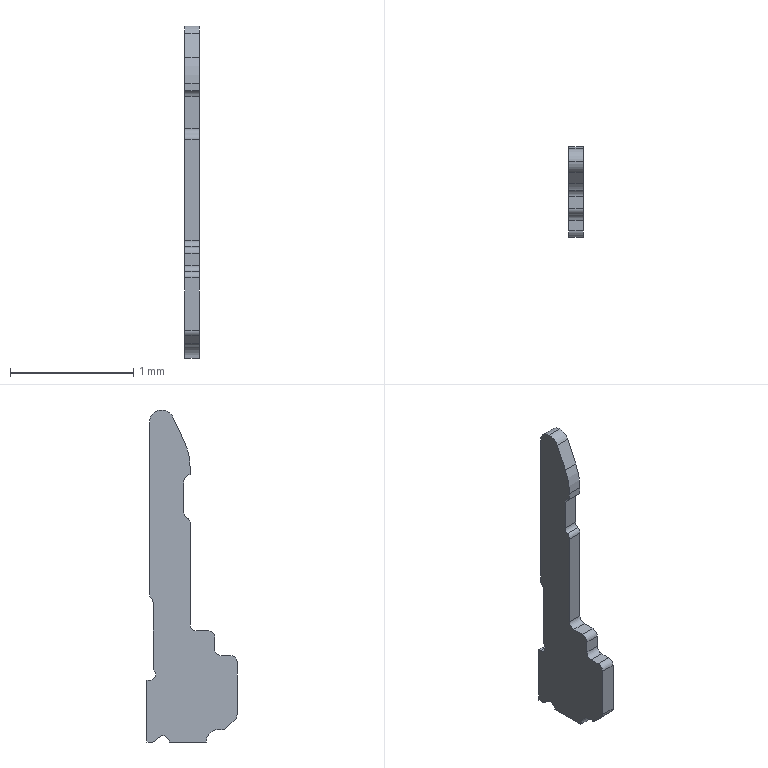Part | Creo | 1 solid | 40 faces | box 0.12 x 0.73 x 2.69 mm | volume 0.132 mm3 | cylinder 20 | plane 20 | commonest cylinder face diameters 0.1 x16 0.2 x3 1 x1
STEP:
#1=CARTESIAN_POINT('',(0.,0.,0.));
#2=DIRECTION('',(0.,0.,1.));
#3=DIRECTION('',(1.,0.,0.));
#4=AXIS2_PLACEMENT_3D('',#1,#2,#3);
#5=CARTESIAN_POINT('',(0.12,978.915,-1855.853));
#6=VERTEX_POINT('',#5);
#7=CARTESIAN_POINT('',(0.12,978.872,-1855.828));
#8=VERTEX_POINT('',#7);
#9=CARTESIAN_POINT('',(0.12,978.872,-1855.878));
#10=DIRECTION('',(1.,0.,0.));
#11=DIRECTION('',(0.,0.866,0.5));
#12=AXIS2_PLACEMENT_3D('',#9,#10,#11);
#13=CIRCLE('',#12,0.05);
#14=EDGE_CURVE('',#6,#8,#13,.T.);
#15=ORIENTED_EDGE('',*,*,#14,.F.);
#16=CARTESIAN_POINT('',(0.,978.915,-1855.853));
#17=VERTEX_POINT('',#16);
#18=CARTESIAN_POINT('',(0.,978.915,-1855.853));
#19=DIRECTION('',(1.,0.,0.));
#20=VECTOR('',#19,0.12);
#21=LINE('',#18,#20);
#22=EDGE_CURVE('',#17,#6,#21,.T.);
#23=ORIENTED_EDGE('',*,*,#22,.F.);
#24=CARTESIAN_POINT('',(0.,978.872,-1855.828));
#25=VERTEX_POINT('',#24);
#26=CARTESIAN_POINT('',(0.,978.872,-1855.878));
#27=DIRECTION('',(-1.,0.,0.));
#28=DIRECTION('',(0.,0.,1.));
#29=AXIS2_PLACEMENT_3D('',#26,#27,#28);
#30=CIRCLE('',#29,0.05);
#31=EDGE_CURVE('',#25,#17,#30,.T.);
#32=ORIENTED_EDGE('',*,*,#31,.F.);
#33=CARTESIAN_POINT('',(0.,978.872,-1855.828));
#34=DIRECTION('',(1.,0.,0.));
#35=VECTOR('',#34,0.12);
#36=LINE('',#33,#35);
#37=EDGE_CURVE('',#25,#8,#36,.T.);
#38=ORIENTED_EDGE('',*,*,#37,.T.);
#39=EDGE_LOOP('',(#15,#23,#32,#38));
#40=FACE_OUTER_BOUND('',#39,.F.);
#41=CARTESIAN_POINT('',(0.12,978.872,-1855.878));
#42=DIRECTION('',(-1.,0.,0.));
#43=DIRECTION('',(0.,0.,1.));
#44=AXIS2_PLACEMENT_3D('',#41,#42,#43);
#45=CYLINDRICAL_SURFACE('',#44,0.05);
#46=ADVANCED_FACE('',(#40),#45,.F.);
#47=CARTESIAN_POINT('',(0.12,978.286,-1855.693));
#48=VERTEX_POINT('',#47);
#49=CARTESIAN_POINT('',(0.12,978.272,-1855.658));
#50=VERTEX_POINT('',#49);
#51=CARTESIAN_POINT('',(0.12,978.322,-1855.658));
#52=DIRECTION('',(-1.,0.,0.));
#53=DIRECTION('',(0.,-0.7071,-0.7071));
#54=AXIS2_PLACEMENT_3D('',#51,#52,#53);
#55=CIRCLE('',#54,0.05);
#56=EDGE_CURVE('',#48,#50,#55,.T.);
#57=ORIENTED_EDGE('',*,*,#56,.T.);
#58=CARTESIAN_POINT('',(0.12,978.272,-1855.228));
#59=VERTEX_POINT('',#58);
#60=CARTESIAN_POINT('',(0.12,978.272,-1855.658));
#61=DIRECTION('',(0.,0.,1.));
#62=VECTOR('',#61,0.4293);
#63=LINE('',#60,#62);
#64=EDGE_CURVE('',#50,#59,#63,.T.);
#65=ORIENTED_EDGE('',*,*,#64,.T.);
#66=CARTESIAN_POINT('',(0.12,978.322,-1855.178));
#67=VERTEX_POINT('',#66);
#68=CARTESIAN_POINT('',(0.12,978.322,-1855.228));
#69=DIRECTION('',(-1.,0.,0.));
#70=DIRECTION('',(0.,-1.,0.));
#71=AXIS2_PLACEMENT_3D('',#68,#69,#70);
#72=CIRCLE('',#71,0.05);
#73=EDGE_CURVE('',#59,#67,#72,.T.);
#74=ORIENTED_EDGE('',*,*,#73,.T.);
#75=CARTESIAN_POINT('',(0.12,978.402,-1855.178));
#76=VERTEX_POINT('',#75);
#77=CARTESIAN_POINT('',(0.12,978.322,-1855.178));
#78=DIRECTION('',(0.,1.,0.));
#79=VECTOR('',#78,0.08);
#80=LINE('',#77,#79);
#81=EDGE_CURVE('',#67,#76,#80,.T.);
#82=ORIENTED_EDGE('',*,*,#81,.T.);
#83=CARTESIAN_POINT('',(0.12,978.452,-1855.128));
#84=VERTEX_POINT('',#83);
#85=CARTESIAN_POINT('',(0.12,978.402,-1855.128));
#86=DIRECTION('',(1.,0.,0.));
#87=DIRECTION('',(0.,0.,-1.));
#88=AXIS2_PLACEMENT_3D('',#85,#86,#87);
#89=CIRCLE('',#88,0.05);
#90=EDGE_CURVE('',#76,#84,#89,.T.);
#91=ORIENTED_EDGE('',*,*,#90,.T.);
#92=CARTESIAN_POINT('',(0.12,978.452,-1855.028));
#93=VERTEX_POINT('',#92);
#94=CARTESIAN_POINT('',(0.12,978.452,-1855.128));
#95=DIRECTION('',(0.,0.,1.));
#96=VECTOR('',#95,0.1);
#97=LINE('',#94,#96);
#98=EDGE_CURVE('',#84,#93,#97,.T.);
#99=ORIENTED_EDGE('',*,*,#98,.T.);
#100=CARTESIAN_POINT('',(0.12,978.502,-1854.978));
#101=VERTEX_POINT('',#100);
#102=CARTESIAN_POINT('',(0.12,978.502,-1855.028));
#103=DIRECTION('',(-1.,0.,0.));
#104=DIRECTION('',(0.,-1.,0.));
#105=AXIS2_PLACEMENT_3D('',#102,#103,#104);
#106=CIRCLE('',#105,0.05);
#107=EDGE_CURVE('',#93,#101,#106,.T.);
#108=ORIENTED_EDGE('',*,*,#107,.T.);
#109=CARTESIAN_POINT('',(0.12,978.602,-1854.978));
#110=VERTEX_POINT('',#109);
#111=CARTESIAN_POINT('',(0.12,978.502,-1854.978));
#112=DIRECTION('',(0.,1.,0.));
#113=VECTOR('',#112,0.1);
#114=LINE('',#111,#113);
#115=EDGE_CURVE('',#101,#110,#114,.T.);
#116=ORIENTED_EDGE('',*,*,#115,.T.);
#117=CARTESIAN_POINT('',(0.12,978.652,-1854.928));
#118=VERTEX_POINT('',#117);
#119=CARTESIAN_POINT('',(0.12,978.602,-1854.928));
#120=DIRECTION('',(1.,0.,0.));
#121=DIRECTION('',(0.,0.,-1.));
#122=AXIS2_PLACEMENT_3D('',#119,#120,#121);
#123=CIRCLE('',#122,0.05);
#124=EDGE_CURVE('',#110,#118,#123,.T.);
#125=ORIENTED_EDGE('',*,*,#124,.T.);
#126=CARTESIAN_POINT('',(0.12,978.652,-1854.108));
#127=VERTEX_POINT('',#126);
#128=CARTESIAN_POINT('',(0.12,978.652,-1854.928));
#129=DIRECTION('',(0.,0.,1.));
#130=VECTOR('',#129,0.82);
#131=LINE('',#128,#130);
#132=EDGE_CURVE('',#118,#127,#131,.T.);
#133=ORIENTED_EDGE('',*,*,#132,.T.);
#134=CARTESIAN_POINT('',(0.12,978.677,-1854.065));
#135=VERTEX_POINT('',#134);
#136=CARTESIAN_POINT('',(0.12,978.702,-1854.108));
#137=DIRECTION('',(-1.,0.,0.));
#138=DIRECTION('',(0.,-1.,0.));
#139=AXIS2_PLACEMENT_3D('',#136,#137,#138);
#140=CIRCLE('',#139,0.05);
#141=EDGE_CURVE('',#127,#135,#140,.T.);
#142=ORIENTED_EDGE('',*,*,#141,.T.);
#143=CARTESIAN_POINT('',(0.12,978.702,-1854.022));
#144=VERTEX_POINT('',#143);
#145=CARTESIAN_POINT('',(0.12,978.652,-1854.022));
#146=DIRECTION('',(1.,0.,0.));
#147=DIRECTION('',(0.,0.5,-0.866));
#148=AXIS2_PLACEMENT_3D('',#145,#146,#147);
#149=CIRCLE('',#148,0.05);
#150=EDGE_CURVE('',#135,#144,#149,.T.);
#151=ORIENTED_EDGE('',*,*,#150,.T.);
#152=CARTESIAN_POINT('',(0.12,978.702,-1853.764));
#153=VERTEX_POINT('',#152);
#154=CARTESIAN_POINT('',(0.12,978.702,-1854.022));
#155=DIRECTION('',(0.,0.,1.));
#156=VECTOR('',#155,0.258);
#157=LINE('',#154,#156);
#158=EDGE_CURVE('',#144,#153,#157,.T.);
#159=ORIENTED_EDGE('',*,*,#158,.T.);
#160=CARTESIAN_POINT('',(0.12,978.652,-1853.714));
#161=VERTEX_POINT('',#160);
#162=CARTESIAN_POINT('',(0.12,978.652,-1853.764));
#163=DIRECTION('',(1.,0.,0.));
#164=DIRECTION('',(0.,1.,0.000000001));
#165=AXIS2_PLACEMENT_3D('',#162,#163,#164);
#166=CIRCLE('',#165,0.05);
#167=EDGE_CURVE('',#153,#161,#166,.T.);
#168=ORIENTED_EDGE('',*,*,#167,.T.);
#169=CARTESIAN_POINT('',(0.12,978.652,-1853.656));
#170=VERTEX_POINT('',#169);
#171=CARTESIAN_POINT('',(0.12,978.652,-1853.714));
#172=DIRECTION('',(0.,0.,1.));
#173=VECTOR('',#172,0.05743);
#174=LINE('',#171,#173);
#175=EDGE_CURVE('',#161,#170,#174,.T.);
#176=ORIENTED_EDGE('',*,*,#175,.T.);
#177=CARTESIAN_POINT('',(0.12,978.698,-1853.445));
#178=VERTEX_POINT('',#177);
#179=CARTESIAN_POINT('',(0.12,979.152,-1853.656));
#180=DIRECTION('',(-1.,0.,0.));
#181=DIRECTION('',(0.,-1.,0.));
#182=AXIS2_PLACEMENT_3D('',#179,#180,#181);
#183=CIRCLE('',#182,0.5);
#184=EDGE_CURVE('',#170,#178,#183,.T.);
#185=ORIENTED_EDGE('',*,*,#184,.T.);
#186=CARTESIAN_POINT('',(0.12,978.791,-1853.247));
#187=VERTEX_POINT('',#186);
#188=CARTESIAN_POINT('',(0.12,978.698,-1853.445));
#189=DIRECTION('',(0.,0.4226,0.9063));
#190=VECTOR('',#189,0.2189);
#191=LINE('',#188,#190);
#192=EDGE_CURVE('',#178,#187,#191,.T.);
#193=ORIENTED_EDGE('',*,*,#192,.T.);
#194=CARTESIAN_POINT('',(0.12,978.882,-1853.189));
#195=VERTEX_POINT('',#194);
#196=CARTESIAN_POINT('',(0.12,978.882,-1853.289));
#197=DIRECTION('',(-1.,0.,0.));
#198=DIRECTION('',(0.,-0.9063,0.4226));
#199=AXIS2_PLACEMENT_3D('',#196,#197,#198);
#200=CIRCLE('',#199,0.1);
#201=EDGE_CURVE('',#187,#195,#200,.T.);
#202=ORIENTED_EDGE('',*,*,#201,.T.);
#203=CARTESIAN_POINT('',(0.12,978.982,-1853.289));
#204=VERTEX_POINT('',#203);
#205=CARTESIAN_POINT('',(0.12,978.882,-1853.289));
#206=DIRECTION('',(-1.,0.,0.));
#207=DIRECTION('',(0.,0.,1.));
#208=AXIS2_PLACEMENT_3D('',#205,#206,#207);
#209=CIRCLE('',#208,0.1);
#210=EDGE_CURVE('',#195,#204,#209,.T.);
#211=ORIENTED_EDGE('',*,*,#210,.T.);
#212=CARTESIAN_POINT('',(0.12,978.982,-1854.678));
#213=VERTEX_POINT('',#212);
#214=CARTESIAN_POINT('',(0.12,978.982,-1853.289));
#215=DIRECTION('',(0.,0.,-1.));
#216=VECTOR('',#215,1.389);
#217=LINE('',#214,#216);
#218=EDGE_CURVE('',#204,#213,#217,.T.);
#219=ORIENTED_EDGE('',*,*,#218,.T.);
#220=CARTESIAN_POINT('',(0.12,978.967,-1854.713));
#221=VERTEX_POINT('',#220);
#222=CARTESIAN_POINT('',(0.12,978.932,-1854.678));
#223=DIRECTION('',(-1.,0.,0.));
#224=DIRECTION('',(0.,1.,0.));
#225=AXIS2_PLACEMENT_3D('',#222,#223,#224);
#226=CIRCLE('',#225,0.05);
#227=EDGE_CURVE('',#213,#221,#226,.T.);
#228=ORIENTED_EDGE('',*,*,#227,.T.);
#229=CARTESIAN_POINT('',(0.12,978.966,-1854.714));
#230=VERTEX_POINT('',#229);
#231=CARTESIAN_POINT('',(0.12,978.967,-1854.713));
#232=DIRECTION('',(0.,-0.7071,-0.7071));
#233=VECTOR('',#232,0.001005);
#234=LINE('',#231,#233);
#235=EDGE_CURVE('',#221,#230,#234,.T.);
#236=ORIENTED_EDGE('',*,*,#235,.T.);
#237=CARTESIAN_POINT('',(0.12,978.952,-1854.749));
#238=VERTEX_POINT('',#237);
#239=CARTESIAN_POINT('',(0.12,979.002,-1854.749));
#240=DIRECTION('',(1.,0.,0.));
#241=DIRECTION('',(0.,-0.7071,0.7071));
#242=AXIS2_PLACEMENT_3D('',#239,#240,#241);
#243=CIRCLE('',#242,0.05);
#244=EDGE_CURVE('',#230,#238,#243,.T.);
#245=ORIENTED_EDGE('',*,*,#244,.T.);
#246=CARTESIAN_POINT('',(0.12,978.952,-1855.267));
#247=VERTEX_POINT('',#246);
#248=CARTESIAN_POINT('',(0.12,978.952,-1854.749));
#249=DIRECTION('',(0.,0.,-1.));
#250=VECTOR('',#249,0.5179);
#251=LINE('',#248,#250);
#252=EDGE_CURVE('',#238,#247,#251,.T.);
#253=ORIENTED_EDGE('',*,*,#252,.T.);
#254=CARTESIAN_POINT('',(0.12,978.945,-1855.292));
#255=VERTEX_POINT('',#254);
#256=CARTESIAN_POINT('',(0.12,978.902,-1855.267));
#257=DIRECTION('',(-1.,0.,0.));
#258=DIRECTION('',(0.,1.,0.));
#259=AXIS2_PLACEMENT_3D('',#256,#257,#258);
#260=CIRCLE('',#259,0.05);
#261=EDGE_CURVE('',#247,#255,#260,.T.);
#262=ORIENTED_EDGE('',*,*,#261,.T.);
#263=CARTESIAN_POINT('',(0.12,978.938,-1855.303));
#264=VERTEX_POINT('',#263);
#265=CARTESIAN_POINT('',(0.12,978.945,-1855.292));
#266=DIRECTION('',(0.,-0.5,-0.866));
#267=VECTOR('',#266,0.01321);
#268=LINE('',#265,#267);
#269=EDGE_CURVE('',#255,#264,#268,.T.);
#270=ORIENTED_EDGE('',*,*,#269,.T.);
#271=CARTESIAN_POINT('',(0.12,978.982,-1855.378));
#272=VERTEX_POINT('',#271);
#273=CARTESIAN_POINT('',(0.12,978.982,-1855.328));
#274=DIRECTION('',(1.,0.,0.));
#275=DIRECTION('',(0.,-0.866,0.5));
#276=AXIS2_PLACEMENT_3D('',#273,#274,#275);
#277=CIRCLE('',#276,0.05);
#278=EDGE_CURVE('',#264,#272,#277,.T.);
#279=ORIENTED_EDGE('',*,*,#278,.T.);
#280=CARTESIAN_POINT('',(0.12,979.002,-1855.378));
#281=VERTEX_POINT('',#280);
#282=CARTESIAN_POINT('',(0.12,978.982,-1855.378));
#283=DIRECTION('',(0.,1.,0.));
#284=VECTOR('',#283,0.02);
#285=LINE('',#282,#284);
#286=EDGE_CURVE('',#272,#281,#285,.T.);
#287=ORIENTED_EDGE('',*,*,#286,.T.);
#288=CARTESIAN_POINT('',(0.12,979.002,-1855.878));
#289=VERTEX_POINT('',#288);
#290=CARTESIAN_POINT('',(0.12,979.002,-1855.378));
#291=DIRECTION('',(0.,0.,-1.));
#292=VECTOR('',#291,0.5);
#293=LINE('',#290,#292);
#294=EDGE_CURVE('',#281,#289,#293,.T.);
#295=ORIENTED_EDGE('',*,*,#294,.T.);
#296=CARTESIAN_POINT('',(0.12,978.958,-1855.878));
#297=VERTEX_POINT('',#296);
#298=CARTESIAN_POINT('',(0.12,979.002,-1855.878));
#299=DIRECTION('',(0.,-1.,0.));
#300=VECTOR('',#299,0.0434);
#301=LINE('',#298,#300);
#302=EDGE_CURVE('',#289,#297,#301,.T.);
#303=ORIENTED_EDGE('',*,*,#302,.T.);
#304=CARTESIAN_POINT('',(0.12,978.958,-1855.828));
#305=DIRECTION('',(-1.,0.,0.));
#306=DIRECTION('',(0.,0.,-1.));
#307=AXIS2_PLACEMENT_3D('',#304,#305,#306);
#308=CIRCLE('',#307,0.05);
#309=EDGE_CURVE('',#297,#6,#308,.T.);
#310=ORIENTED_EDGE('',*,*,#309,.T.);
#311=ORIENTED_EDGE('',*,*,#14,.T.);
#312=CARTESIAN_POINT('',(0.12,978.822,-1855.878));
#313=VERTEX_POINT('',#312);
#314=CARTESIAN_POINT('',(0.12,978.872,-1855.878));
#315=DIRECTION('',(1.,0.,0.));
#316=DIRECTION('',(0.,0.,1.));
#317=AXIS2_PLACEMENT_3D('',#314,#315,#316);
#318=CIRCLE('',#317,0.05);
#319=EDGE_CURVE('',#8,#313,#318,.T.);
#320=ORIENTED_EDGE('',*,*,#319,.T.);
#321=CARTESIAN_POINT('',(0.12,978.522,-1855.878));
#322=VERTEX_POINT('',#321);
#323=CARTESIAN_POINT('',(0.12,978.822,-1855.878));
#324=DIRECTION('',(0.,-1.,0.));
#325=VECTOR('',#324,0.3);
#326=LINE('',#323,#325);
#327=EDGE_CURVE('',#313,#322,#326,.T.);
#328=ORIENTED_EDGE('',*,*,#327,.T.);
#329=CARTESIAN_POINT('',(0.12,978.422,-1855.778));
#330=VERTEX_POINT('',#329);
#331=CARTESIAN_POINT('',(0.12,978.422,-1855.878));
#332=DIRECTION('',(1.,0.,0.));
#333=DIRECTION('',(0.,1.,0.));
#334=AXIS2_PLACEMENT_3D('',#331,#332,#333);
#335=CIRCLE('',#334,0.1);
#336=EDGE_CURVE('',#322,#330,#335,.T.);
#337=ORIENTED_EDGE('',*,*,#336,.T.);
#338=CARTESIAN_POINT('',(0.12,978.392,-1855.778));
#339=VERTEX_POINT('',#338);
#340=CARTESIAN_POINT('',(0.12,978.422,-1855.778));
#341=DIRECTION('',(0.,-1.,0.));
#342=VECTOR('',#341,0.02929);
#343=LINE('',#340,#342);
#344=EDGE_CURVE('',#330,#339,#343,.T.);
#345=ORIENTED_EDGE('',*,*,#344,.T.);
#346=CARTESIAN_POINT('',(0.12,978.357,-1855.764));
#347=VERTEX_POINT('',#346);
#348=CARTESIAN_POINT('',(0.12,978.392,-1855.728));
#349=DIRECTION('',(-1.,0.,0.));
#350=DIRECTION('',(0.,0.,-1.));
#351=AXIS2_PLACEMENT_3D('',#348,#349,#350);
#352=CIRCLE('',#351,0.05);
#353=EDGE_CURVE('',#339,#347,#352,.T.);
#354=ORIENTED_EDGE('',*,*,#353,.T.);
#355=CARTESIAN_POINT('',(0.12,978.357,-1855.764));
#356=DIRECTION('',(0.,-0.7071,0.7071));
#357=VECTOR('',#356,0.1);
#358=LINE('',#355,#357);
#359=EDGE_CURVE('',#347,#48,#358,.T.);
#360=ORIENTED_EDGE('',*,*,#359,.T.);
#361=EDGE_LOOP('',(#57,#65,#74,#82,#91,#99,#108,#116,#125,#133,#142,#151,#159,#168,#176,#185,#193,#202,#211,#219,#228,#236,#245,#253,#262,#270,#279,#287,#295,#303,#310,#311,#320,#328,#337,#345,#354,#360));
#362=FACE_OUTER_BOUND('',#361,.F.);
#363=CARTESIAN_POINT('',(0.12,978.322,-1855.658));
#364=DIRECTION('',(1.,0.,0.));
#365=DIRECTION('',(0.,0.,-1.));
#366=AXIS2_PLACEMENT_3D('',#363,#364,#365);
#367=PLANE('',#366);
#368=ADVANCED_FACE('',(#362),#367,.T.);
#369=CARTESIAN_POINT('',(0.,978.272,-1855.658));
#370=VERTEX_POINT('',#369);
#371=CARTESIAN_POINT('',(0.,978.286,-1855.693));
#372=VERTEX_POINT('',#371);
#373=CARTESIAN_POINT('',(0.,978.322,-1855.658));
#374=DIRECTION('',(1.,0.,0.));
#375=DIRECTION('',(0.,-1.,0.));
#376=AXIS2_PLACEMENT_3D('',#373,#374,#375);
#377=CIRCLE('',#376,0.05);
#378=EDGE_CURVE('',#370,#372,#377,.T.);
#379=ORIENTED_EDGE('',*,*,#378,.F.);
#380=CARTESIAN_POINT('',(0.,978.272,-1855.658));
#381=DIRECTION('',(1.,0.,0.));
#382=VECTOR('',#381,0.12);
#383=LINE('',#380,#382);
#384=EDGE_CURVE('',#370,#50,#383,.T.);
#385=ORIENTED_EDGE('',*,*,#384,.T.);
#386=ORIENTED_EDGE('',*,*,#56,.F.);
#387=CARTESIAN_POINT('',(0.12,978.286,-1855.693));
#388=DIRECTION('',(-1.,0.000000006,-0.000000006));
#389=VECTOR('',#388,0.12);
#390=LINE('',#387,#389);
#391=EDGE_CURVE('',#48,#372,#390,.T.);
#392=ORIENTED_EDGE('',*,*,#391,.T.);
#393=EDGE_LOOP('',(#379,#385,#386,#392));
#394=FACE_OUTER_BOUND('',#393,.F.);
#395=CARTESIAN_POINT('',(0.12,978.322,-1855.658));
#396=DIRECTION('',(-1.,0.,0.));
#397=DIRECTION('',(0.,0.,1.));
#398=AXIS2_PLACEMENT_3D('',#395,#396,#397);
#399=CYLINDRICAL_SURFACE('',#398,0.05);
#400=ADVANCED_FACE('',(#394),#399,.T.);
#401=ORIENTED_EDGE('',*,*,#378,.T.);
#402=CARTESIAN_POINT('',(0.,978.357,-1855.764));
#403=VERTEX_POINT('',#402);
#404=CARTESIAN_POINT('',(0.,978.286,-1855.693));
#405=DIRECTION('',(0.,0.7071,-0.7071));
#406=VECTOR('',#405,0.1);
#407=LINE('',#404,#406);
#408=EDGE_CURVE('',#372,#403,#407,.T.);
#409=ORIENTED_EDGE('',*,*,#408,.T.);
#410=CARTESIAN_POINT('',(0.,978.392,-1855.778));
#411=VERTEX_POINT('',#410);
#412=CARTESIAN_POINT('',(0.,978.392,-1855.728));
#413=DIRECTION('',(1.,0.,0.));
#414=DIRECTION('',(0.,-0.7071,-0.7071));
#415=AXIS2_PLACEMENT_3D('',#412,#413,#414);
#416=CIRCLE('',#415,0.05);
#417=EDGE_CURVE('',#403,#411,#416,.T.);
#418=ORIENTED_EDGE('',*,*,#417,.T.);
#419=CARTESIAN_POINT('',(0.,978.422,-1855.778));
#420=VERTEX_POINT('',#419);
#421=CARTESIAN_POINT('',(0.,978.422,-1855.778));
#422=DIRECTION('',(0.,-1.,0.));
#423=VECTOR('',#422,0.02929);
#424=LINE('',#421,#423);
#425=EDGE_CURVE('',#420,#411,#424,.T.);
#426=ORIENTED_EDGE('',*,*,#425,.F.);
#427=CARTESIAN_POINT('',(0.,978.522,-1855.878));
#428=VERTEX_POINT('',#427);
#429=CARTESIAN_POINT('',(0.,978.422,-1855.878));
#430=DIRECTION('',(-1.,0.,0.));
#431=DIRECTION('',(0.,0.,1.));
#432=AXIS2_PLACEMENT_3D('',#429,#430,#431);
#433=CIRCLE('',#432,0.1);
#434=EDGE_CURVE('',#420,#428,#433,.T.);
#435=ORIENTED_EDGE('',*,*,#434,.T.);
#436=CARTESIAN_POINT('',(0.,978.822,-1855.878));
#437=VERTEX_POINT('',#436);
#438=CARTESIAN_POINT('',(0.,978.822,-1855.878));
#439=DIRECTION('',(0.,-1.,0.));
#440=VECTOR('',#439,0.3);
#441=LINE('',#438,#440);
#442=EDGE_CURVE('',#437,#428,#441,.T.);
#443=ORIENTED_EDGE('',*,*,#442,.F.);
#444=CARTESIAN_POINT('',(0.,978.872,-1855.878));
#445=DIRECTION('',(-1.,0.,0.));
#446=DIRECTION('',(0.,-1.,0.));
#447=AXIS2_PLACEMENT_3D('',#444,#445,#446);
#448=CIRCLE('',#447,0.05);
#449=EDGE_CURVE('',#437,#25,#448,.T.);
#450=ORIENTED_EDGE('',*,*,#449,.T.);
#451=ORIENTED_EDGE('',*,*,#31,.T.);
#452=CARTESIAN_POINT('',(0.,978.958,-1855.878));
#453=VERTEX_POINT('',#452);
#454=CARTESIAN_POINT('',(0.,978.958,-1855.828));
#455=DIRECTION('',(1.,0.,0.));
#456=DIRECTION('',(0.,-0.866,-0.5));
#457=AXIS2_PLACEMENT_3D('',#454,#455,#456);
#458=CIRCLE('',#457,0.05);
#459=EDGE_CURVE('',#17,#453,#458,.T.);
#460=ORIENTED_EDGE('',*,*,#459,.T.);
#461=CARTESIAN_POINT('',(0.,979.002,-1855.878));
#462=VERTEX_POINT('',#461);
#463=CARTESIAN_POINT('',(0.,979.002,-1855.878));
#464=DIRECTION('',(0.,-1.,0.));
#465=VECTOR('',#464,0.0434);
#466=LINE('',#463,#465);
#467=EDGE_CURVE('',#462,#453,#466,.T.);
#468=ORIENTED_EDGE('',*,*,#467,.F.);
#469=CARTESIAN_POINT('',(0.,979.002,-1855.378));
#470=VERTEX_POINT('',#469);
#471=CARTESIAN_POINT('',(0.,979.002,-1855.378));
#472=DIRECTION('',(0.,0.,-1.));
#473=VECTOR('',#472,0.5);
#474=LINE('',#471,#473);
#475=EDGE_CURVE('',#470,#462,#474,.T.);
#476=ORIENTED_EDGE('',*,*,#475,.F.);
#477=CARTESIAN_POINT('',(0.,978.982,-1855.378));
#478=VERTEX_POINT('',#477);
#479=CARTESIAN_POINT('',(0.,978.982,-1855.378));
#480=DIRECTION('',(0.,1.,0.));
#481=VECTOR('',#480,0.02);
#482=LINE('',#479,#481);
#483=EDGE_CURVE('',#478,#470,#482,.T.);
#484=ORIENTED_EDGE('',*,*,#483,.F.);
#485=CARTESIAN_POINT('',(0.,978.938,-1855.303));
#486=VERTEX_POINT('',#485);
#487=CARTESIAN_POINT('',(0.,978.982,-1855.328));
#488=DIRECTION('',(-1.,0.,0.));
#489=DIRECTION('',(0.,0.,-1.));
#490=AXIS2_PLACEMENT_3D('',#487,#488,#489);
#491=CIRCLE('',#490,0.05);
#492=EDGE_CURVE('',#478,#486,#491,.T.);
#493=ORIENTED_EDGE('',*,*,#492,.T.);
#494=CARTESIAN_POINT('',(0.,978.945,-1855.292));
#495=VERTEX_POINT('',#494);
#496=CARTESIAN_POINT('',(0.,978.938,-1855.303));
#497=DIRECTION('',(0.,0.5,0.866));
#498=VECTOR('',#497,0.01321);
#499=LINE('',#496,#498);
#500=EDGE_CURVE('',#486,#495,#499,.T.);
#501=ORIENTED_EDGE('',*,*,#500,.T.);
#502=CARTESIAN_POINT('',(0.,978.952,-1855.267));
#503=VERTEX_POINT('',#502);
#504=CARTESIAN_POINT('',(0.,978.902,-1855.267));
#505=DIRECTION('',(1.,0.,0.));
#506=DIRECTION('',(0.,0.866,-0.5));
#507=AXIS2_PLACEMENT_3D('',#504,#505,#506);
#508=CIRCLE('',#507,0.05);
#509=EDGE_CURVE('',#495,#503,#508,.T.);
#510=ORIENTED_EDGE('',*,*,#509,.T.);
#511=CARTESIAN_POINT('',(0.,978.952,-1854.749));
#512=VERTEX_POINT('',#511);
#513=CARTESIAN_POINT('',(0.,978.952,-1854.749));
#514=DIRECTION('',(0.,0.,-1.));
#515=VECTOR('',#514,0.5179);
#516=LINE('',#513,#515);
#517=EDGE_CURVE('',#512,#503,#516,.T.);
#518=ORIENTED_EDGE('',*,*,#517,.F.);
#519=CARTESIAN_POINT('',(0.,978.966,-1854.714));
#520=VERTEX_POINT('',#519);
#521=CARTESIAN_POINT('',(0.,979.002,-1854.749));
#522=DIRECTION('',(-1.,0.,0.));
#523=DIRECTION('',(0.,-1.,0.));
#524=AXIS2_PLACEMENT_3D('',#521,#522,#523);
#525=CIRCLE('',#524,0.05);
#526=EDGE_CURVE('',#512,#520,#525,.T.);
#527=ORIENTED_EDGE('',*,*,#526,.T.);
#528=CARTESIAN_POINT('',(0.,978.967,-1854.713));
#529=VERTEX_POINT('',#528);
#530=CARTESIAN_POINT('',(0.,978.966,-1854.714));
#531=DIRECTION('',(0.,0.7071,0.7071));
#532=VECTOR('',#531,0.001005);
#533=LINE('',#530,#532);
#534=EDGE_CURVE('',#520,#529,#533,.T.);
#535=ORIENTED_EDGE('',*,*,#534,.T.);
#536=CARTESIAN_POINT('',(0.,978.982,-1854.678));
#537=VERTEX_POINT('',#536);
#538=CARTESIAN_POINT('',(0.,978.932,-1854.678));
#539=DIRECTION('',(1.,0.,0.));
#540=DIRECTION('',(0.,0.7071,-0.7071));
#541=AXIS2_PLACEMENT_3D('',#538,#539,#540);
#542=CIRCLE('',#541,0.05);
#543=EDGE_CURVE('',#529,#537,#542,.T.);
#544=ORIENTED_EDGE('',*,*,#543,.T.);
#545=CARTESIAN_POINT('',(0.,978.982,-1853.289));
#546=VERTEX_POINT('',#545);
#547=CARTESIAN_POINT('',(0.,978.982,-1853.289));
#548=DIRECTION('',(0.,0.,-1.));
#549=VECTOR('',#548,1.389);
#550=LINE('',#547,#549);
#551=EDGE_CURVE('',#546,#537,#550,.T.);
#552=ORIENTED_EDGE('',*,*,#551,.F.);
#553=CARTESIAN_POINT('',(0.,978.882,-1853.189));
#554=VERTEX_POINT('',#553);
#555=CARTESIAN_POINT('',(0.,978.882,-1853.289));
#556=DIRECTION('',(1.,0.,0.));
#557=DIRECTION('',(0.,1.,0.));
#558=AXIS2_PLACEMENT_3D('',#555,#556,#557);
#559=CIRCLE('',#558,0.1);
#560=EDGE_CURVE('',#546,#554,#559,.T.);
#561=ORIENTED_EDGE('',*,*,#560,.T.);
#562=CARTESIAN_POINT('',(0.,978.791,-1853.247));
#563=VERTEX_POINT('',#562);
#564=CARTESIAN_POINT('',(0.,978.882,-1853.289));
#565=DIRECTION('',(1.,0.,0.));
#566=DIRECTION('',(0.,0.,1.));
#567=AXIS2_PLACEMENT_3D('',#564,#565,#566);
#568=CIRCLE('',#567,0.1);
#569=EDGE_CURVE('',#554,#563,#568,.T.);
#570=ORIENTED_EDGE('',*,*,#569,.T.);
#571=CARTESIAN_POINT('',(0.,978.698,-1853.445));
#572=VERTEX_POINT('',#571);
#573=CARTESIAN_POINT('',(0.,978.791,-1853.247));
#574=DIRECTION('',(0.,-0.4226,-0.9063));
#575=VECTOR('',#574,0.2189);
#576=LINE('',#573,#575);
#577=EDGE_CURVE('',#563,#572,#576,.T.);
#578=ORIENTED_EDGE('',*,*,#577,.T.);
#579=CARTESIAN_POINT('',(0.,978.652,-1853.656));
#580=VERTEX_POINT('',#579);
#581=CARTESIAN_POINT('',(0.,979.152,-1853.656));
#582=DIRECTION('',(1.,0.,0.));
#583=DIRECTION('',(0.,-0.9063,0.4226));
#584=AXIS2_PLACEMENT_3D('',#581,#582,#583);
#585=CIRCLE('',#584,0.5);
#586=EDGE_CURVE('',#572,#580,#585,.T.);
#587=ORIENTED_EDGE('',*,*,#586,.T.);
#588=CARTESIAN_POINT('',(0.,978.652,-1853.714));
#589=VERTEX_POINT('',#588);
#590=CARTESIAN_POINT('',(0.,978.652,-1853.714));
#591=DIRECTION('',(0.,0.,1.));
#592=VECTOR('',#591,0.05743);
#593=LINE('',#590,#592);
#594=EDGE_CURVE('',#589,#580,#593,.T.);
#595=ORIENTED_EDGE('',*,*,#594,.F.);
#596=CARTESIAN_POINT('',(0.,978.702,-1853.764));
#597=VERTEX_POINT('',#596);
#598=CARTESIAN_POINT('',(0.,978.652,-1853.764));
#599=DIRECTION('',(-1.,0.,0.));
#600=DIRECTION('',(0.,0.,1.));
#601=AXIS2_PLACEMENT_3D('',#598,#599,#600);
#602=CIRCLE('',#601,0.05);
#603=EDGE_CURVE('',#589,#597,#602,.T.);
#604=ORIENTED_EDGE('',*,*,#603,.T.);
#605=CARTESIAN_POINT('',(0.,978.702,-1854.022));
#606=VERTEX_POINT('',#605);
#607=CARTESIAN_POINT('',(0.,978.702,-1854.022));
#608=DIRECTION('',(0.,0.,1.));
#609=VECTOR('',#608,0.258);
#610=LINE('',#607,#609);
#611=EDGE_CURVE('',#606,#597,#610,.T.);
#612=ORIENTED_EDGE('',*,*,#611,.F.);
#613=CARTESIAN_POINT('',(0.,978.677,-1854.065));
#614=VERTEX_POINT('',#613);
#615=CARTESIAN_POINT('',(0.,978.652,-1854.022));
#616=DIRECTION('',(-1.,0.,0.));
#617=DIRECTION('',(0.,1.,0.000000034));
#618=AXIS2_PLACEMENT_3D('',#615,#616,#617);
#619=CIRCLE('',#618,0.05);
#620=EDGE_CURVE('',#606,#614,#619,.T.);
#621=ORIENTED_EDGE('',*,*,#620,.T.);
#622=CARTESIAN_POINT('',(0.,978.652,-1854.108));
#623=VERTEX_POINT('',#622);
#624=CARTESIAN_POINT('',(0.,978.702,-1854.108));
#625=DIRECTION('',(1.,0.,0.));
#626=DIRECTION('',(0.,-0.5,0.866));
#627=AXIS2_PLACEMENT_3D('',#624,#625,#626);
#628=CIRCLE('',#627,0.05);
#629=EDGE_CURVE('',#614,#623,#628,.T.);
#630=ORIENTED_EDGE('',*,*,#629,.T.);
#631=CARTESIAN_POINT('',(0.,978.652,-1854.928));
#632=VERTEX_POINT('',#631);
#633=CARTESIAN_POINT('',(0.,978.652,-1854.928));
#634=DIRECTION('',(0.,0.,1.));
#635=VECTOR('',#634,0.82);
#636=LINE('',#633,#635);
#637=EDGE_CURVE('',#632,#623,#636,.T.);
#638=ORIENTED_EDGE('',*,*,#637,.F.);
#639=CARTESIAN_POINT('',(0.,978.602,-1854.978));
#640=VERTEX_POINT('',#639);
#641=CARTESIAN_POINT('',(0.,978.602,-1854.928));
#642=DIRECTION('',(-1.,0.,0.));
#643=DIRECTION('',(0.,1.,0.));
#644=AXIS2_PLACEMENT_3D('',#641,#642,#643);
#645=CIRCLE('',#644,0.05);
#646=EDGE_CURVE('',#632,#640,#645,.T.);
#647=ORIENTED_EDGE('',*,*,#646,.T.);
#648=CARTESIAN_POINT('',(0.,978.502,-1854.978));
#649=VERTEX_POINT('',#648);
#650=CARTESIAN_POINT('',(0.,978.502,-1854.978));
#651=DIRECTION('',(0.,1.,0.));
#652=VECTOR('',#651,0.1);
#653=LINE('',#650,#652);
#654=EDGE_CURVE('',#649,#640,#653,.T.);
#655=ORIENTED_EDGE('',*,*,#654,.F.);
#656=CARTESIAN_POINT('',(0.,978.452,-1855.028));
#657=VERTEX_POINT('',#656);
#658=CARTESIAN_POINT('',(0.,978.502,-1855.028));
#659=DIRECTION('',(1.,0.,0.));
#660=DIRECTION('',(0.,0.,1.));
#661=AXIS2_PLACEMENT_3D('',#658,#659,#660);
#662=CIRCLE('',#661,0.05);
#663=EDGE_CURVE('',#649,#657,#662,.T.);
#664=ORIENTED_EDGE('',*,*,#663,.T.);
#665=CARTESIAN_POINT('',(0.,978.452,-1855.128));
#666=VERTEX_POINT('',#665);
#667=CARTESIAN_POINT('',(0.,978.452,-1855.128));
#668=DIRECTION('',(0.,0.,1.));
#669=VECTOR('',#668,0.1);
#670=LINE('',#667,#669);
#671=EDGE_CURVE('',#666,#657,#670,.T.);
#672=ORIENTED_EDGE('',*,*,#671,.F.);
#673=CARTESIAN_POINT('',(0.,978.402,-1855.178));
#674=VERTEX_POINT('',#673);
#675=CARTESIAN_POINT('',(0.,978.402,-1855.128));
#676=DIRECTION('',(-1.,0.,0.));
#677=DIRECTION('',(0.,1.,0.));
#678=AXIS2_PLACEMENT_3D('',#675,#676,#677);
#679=CIRCLE('',#678,0.05);
#680=EDGE_CURVE('',#666,#674,#679,.T.);
#681=ORIENTED_EDGE('',*,*,#680,.T.);
#682=CARTESIAN_POINT('',(0.,978.322,-1855.178));
#683=VERTEX_POINT('',#682);
#684=CARTESIAN_POINT('',(0.,978.322,-1855.178));
#685=DIRECTION('',(0.,1.,0.));
#686=VECTOR('',#685,0.08);
#687=LINE('',#684,#686);
#688=EDGE_CURVE('',#683,#674,#687,.T.);
#689=ORIENTED_EDGE('',*,*,#688,.F.);
#690=CARTESIAN_POINT('',(0.,978.272,-1855.228));
#691=VERTEX_POINT('',#690);
#692=CARTESIAN_POINT('',(0.,978.322,-1855.228));
#693=DIRECTION('',(1.,0.,0.));
#694=DIRECTION('',(0.,0.,1.));
#695=AXIS2_PLACEMENT_3D('',#692,#693,#694);
#696=CIRCLE('',#695,0.05);
#697=EDGE_CURVE('',#683,#691,#696,.T.);
#698=ORIENTED_EDGE('',*,*,#697,.T.);
#699=CARTESIAN_POINT('',(0.,978.272,-1855.658));
#700=DIRECTION('',(0.,0.,1.));
#701=VECTOR('',#700,0.4293);
#702=LINE('',#699,#701);
#703=EDGE_CURVE('',#370,#691,#702,.T.);
#704=ORIENTED_EDGE('',*,*,#703,.F.);
#705=EDGE_LOOP('',(#401,#409,#418,#426,#435,#443,#450,#451,#460,#468,#476,#484,#493,#501,#510,#518,#527,#535,#544,#552,#561,#570,#578,#587,#595,#604,#612,#621,#630,#638,#647,#655,#664,#672,#681,#689,#698,#704));
#706=FACE_OUTER_BOUND('',#705,.F.);
#707=CARTESIAN_POINT('',(0.,978.322,-1855.658));
#708=DIRECTION('',(1.,0.,0.));
#709=DIRECTION('',(0.,0.,-1.));
#710=AXIS2_PLACEMENT_3D('',#707,#708,#709);
#711=PLANE('',#710);
#712=ADVANCED_FACE('',(#706),#711,.F.);
#713=ORIENTED_EDGE('',*,*,#408,.F.);
#714=ORIENTED_EDGE('',*,*,#391,.F.);
#715=ORIENTED_EDGE('',*,*,#359,.F.);
#716=CARTESIAN_POINT('',(0.,978.357,-1855.764));
#717=DIRECTION('',(1.,0.000000007,-0.000000007));
#718=VECTOR('',#717,0.12);
#719=LINE('',#716,#718);
#720=EDGE_CURVE('',#403,#347,#719,.T.);
#721=ORIENTED_EDGE('',*,*,#720,.F.);
#722=EDGE_LOOP('',(#713,#714,#715,#721));
#723=FACE_OUTER_BOUND('',#722,.F.);
#724=CARTESIAN_POINT('',(0.12,978.357,-1855.764));
#725=DIRECTION('',(0.,0.7071,0.7071));
#726=DIRECTION('',(0.,-0.7071,0.7071));
#727=AXIS2_PLACEMENT_3D('',#724,#725,#726);
#728=PLANE('',#727);
#729=ADVANCED_FACE('',(#723),#728,.F.);
#730=ORIENTED_EDGE('',*,*,#417,.F.);
#731=ORIENTED_EDGE('',*,*,#720,.T.);
#732=ORIENTED_EDGE('',*,*,#353,.F.);
#733=CARTESIAN_POINT('',(0.12,978.392,-1855.778));
#734=DIRECTION('',(-1.,0.,0.));
#735=VECTOR('',#734,0.12);
#736=LINE('',#733,#735);
#737=EDGE_CURVE('',#339,#411,#736,.T.);
#738=ORIENTED_EDGE('',*,*,#737,.T.);
#739=EDGE_LOOP('',(#730,#731,#732,#738));
#740=FACE_OUTER_BOUND('',#739,.F.);
#741=CARTESIAN_POINT('',(0.12,978.392,-1855.728));
#742=DIRECTION('',(-1.,0.,0.));
#743=DIRECTION('',(0.,0.,1.));
#744=AXIS2_PLACEMENT_3D('',#741,#742,#743);
#745=CYLINDRICAL_SURFACE('',#744,0.05);
#746=ADVANCED_FACE('',(#740),#745,.T.);
#747=ORIENTED_EDGE('',*,*,#425,.T.);
#748=ORIENTED_EDGE('',*,*,#737,.F.);
#749=ORIENTED_EDGE('',*,*,#344,.F.);
#750=CARTESIAN_POINT('',(0.,978.422,-1855.778));
#751=DIRECTION('',(1.,0.,0.));
#752=VECTOR('',#751,0.12);
#753=LINE('',#750,#752);
#754=EDGE_CURVE('',#420,#330,#753,.T.);
#755=ORIENTED_EDGE('',*,*,#754,.F.);
#756=EDGE_LOOP('',(#747,#748,#749,#755));
#757=FACE_OUTER_BOUND('',#756,.F.);
#758=CARTESIAN_POINT('',(0.12,978.392,-1855.778));
#759=DIRECTION('',(0.,0.,1.));
#760=DIRECTION('',(1.,0.,0.));
#761=AXIS2_PLACEMENT_3D('',#758,#759,#760);
#762=PLANE('',#761);
#763=ADVANCED_FACE('',(#757),#762,.F.);
#764=ORIENTED_EDGE('',*,*,#434,.F.);
#765=ORIENTED_EDGE('',*,*,#754,.T.);
#766=ORIENTED_EDGE('',*,*,#336,.F.);
#767=CARTESIAN_POINT('',(0.12,978.522,-1855.878));
#768=DIRECTION('',(-1.,0.,0.));
#769=VECTOR('',#768,0.12);
#770=LINE('',#767,#769);
#771=EDGE_CURVE('',#322,#428,#770,.T.);
#772=ORIENTED_EDGE('',*,*,#771,.T.);
#773=EDGE_LOOP('',(#764,#765,#766,#772));
#774=FACE_OUTER_BOUND('',#773,.F.);
#775=CARTESIAN_POINT('',(0.12,978.422,-1855.878));
#776=DIRECTION('',(-1.,0.,0.));
#777=DIRECTION('',(0.,0.,1.));
#778=AXIS2_PLACEMENT_3D('',#775,#776,#777);
#779=CYLINDRICAL_SURFACE('',#778,0.1);
#780=ADVANCED_FACE('',(#774),#779,.F.);
#781=ORIENTED_EDGE('',*,*,#442,.T.);
#782=ORIENTED_EDGE('',*,*,#771,.F.);
#783=ORIENTED_EDGE('',*,*,#327,.F.);
#784=CARTESIAN_POINT('',(0.,978.822,-1855.878));
#785=DIRECTION('',(1.,0.,0.));
#786=VECTOR('',#785,0.12);
#787=LINE('',#784,#786);
#788=EDGE_CURVE('',#437,#313,#787,.T.);
#789=ORIENTED_EDGE('',*,*,#788,.F.);
#790=EDGE_LOOP('',(#781,#782,#783,#789));
#791=FACE_OUTER_BOUND('',#790,.F.);
#792=CARTESIAN_POINT('',(0.12,978.522,-1855.878));
#793=DIRECTION('',(0.,0.,1.));
#794=DIRECTION('',(1.,0.,0.));
#795=AXIS2_PLACEMENT_3D('',#792,#793,#794);
#796=PLANE('',#795);
#797=ADVANCED_FACE('',(#791),#796,.F.);
#798=ORIENTED_EDGE('',*,*,#37,.F.);
#799=ORIENTED_EDGE('',*,*,#449,.F.);
#800=ORIENTED_EDGE('',*,*,#788,.T.);
#801=ORIENTED_EDGE('',*,*,#319,.F.);
#802=EDGE_LOOP('',(#798,#799,#800,#801));
#803=FACE_OUTER_BOUND('',#802,.F.);
#804=CARTESIAN_POINT('',(0.12,978.872,-1855.878));
#805=DIRECTION('',(-1.,0.,0.));
#806=DIRECTION('',(0.,0.,1.));
#807=AXIS2_PLACEMENT_3D('',#804,#805,#806);
#808=CYLINDRICAL_SURFACE('',#807,0.05);
#809=ADVANCED_FACE('',(#803),#808,.F.);
#810=ORIENTED_EDGE('',*,*,#459,.F.);
#811=ORIENTED_EDGE('',*,*,#22,.T.);
#812=ORIENTED_EDGE('',*,*,#309,.F.);
#813=CARTESIAN_POINT('',(0.12,978.958,-1855.878));
#814=DIRECTION('',(-1.,0.,0.));
#815=VECTOR('',#814,0.12);
#816=LINE('',#813,#815);
#817=EDGE_CURVE('',#297,#453,#816,.T.);
#818=ORIENTED_EDGE('',*,*,#817,.T.);
#819=EDGE_LOOP('',(#810,#811,#812,#818));
#820=FACE_OUTER_BOUND('',#819,.F.);
#821=CARTESIAN_POINT('',(0.12,978.958,-1855.828));
#822=DIRECTION('',(-1.,0.,0.));
#823=DIRECTION('',(0.,0.,1.));
#824=AXIS2_PLACEMENT_3D('',#821,#822,#823);
#825=CYLINDRICAL_SURFACE('',#824,0.05);
#826=ADVANCED_FACE('',(#820),#825,.T.);
#827=ORIENTED_EDGE('',*,*,#467,.T.);
#828=ORIENTED_EDGE('',*,*,#817,.F.);
#829=ORIENTED_EDGE('',*,*,#302,.F.);
#830=CARTESIAN_POINT('',(0.,979.002,-1855.878));
#831=DIRECTION('',(1.,0.,0.));
#832=VECTOR('',#831,0.12);
#833=LINE('',#830,#832);
#834=EDGE_CURVE('',#462,#289,#833,.T.);
#835=ORIENTED_EDGE('',*,*,#834,.F.);
#836=EDGE_LOOP('',(#827,#828,#829,#835));
#837=FACE_OUTER_BOUND('',#836,.F.);
#838=CARTESIAN_POINT('',(0.12,978.958,-1855.878));
#839=DIRECTION('',(0.,0.,1.));
#840=DIRECTION('',(1.,0.,0.));
#841=AXIS2_PLACEMENT_3D('',#838,#839,#840);
#842=PLANE('',#841);
#843=ADVANCED_FACE('',(#837),#842,.F.);
#844=ORIENTED_EDGE('',*,*,#475,.T.);
#845=ORIENTED_EDGE('',*,*,#834,.T.);
#846=ORIENTED_EDGE('',*,*,#294,.F.);
#847=CARTESIAN_POINT('',(0.,979.002,-1855.378));
#848=DIRECTION('',(1.,0.,0.));
#849=VECTOR('',#848,0.12);
#850=LINE('',#847,#849);
#851=EDGE_CURVE('',#470,#281,#850,.T.);
#852=ORIENTED_EDGE('',*,*,#851,.F.);
#853=EDGE_LOOP('',(#844,#845,#846,#852));
#854=FACE_OUTER_BOUND('',#853,.F.);
#855=CARTESIAN_POINT('',(0.12,979.002,-1855.378));
#856=DIRECTION('',(0.,-1.,0.));
#857=DIRECTION('',(0.,0.,-1.));
#858=AXIS2_PLACEMENT_3D('',#855,#856,#857);
#859=PLANE('',#858);
#860=ADVANCED_FACE('',(#854),#859,.F.);
#861=ORIENTED_EDGE('',*,*,#483,.T.);
#862=ORIENTED_EDGE('',*,*,#851,.T.);
#863=ORIENTED_EDGE('',*,*,#286,.F.);
#864=CARTESIAN_POINT('',(0.,978.982,-1855.378));
#865=DIRECTION('',(1.,0.,0.));
#866=VECTOR('',#865,0.12);
#867=LINE('',#864,#866);
#868=EDGE_CURVE('',#478,#272,#867,.T.);
#869=ORIENTED_EDGE('',*,*,#868,.F.);
#870=EDGE_LOOP('',(#861,#862,#863,#869));
#871=FACE_OUTER_BOUND('',#870,.F.);
#872=CARTESIAN_POINT('',(0.12,978.982,-1855.378));
#873=DIRECTION('',(0.,0.,-1.));
#874=DIRECTION('',(-1.,0.,0.));
#875=AXIS2_PLACEMENT_3D('',#872,#873,#874);
#876=PLANE('',#875);
#877=ADVANCED_FACE('',(#871),#876,.F.);
#878=ORIENTED_EDGE('',*,*,#492,.F.);
#879=ORIENTED_EDGE('',*,*,#868,.T.);
#880=ORIENTED_EDGE('',*,*,#278,.F.);
#881=CARTESIAN_POINT('',(0.12,978.938,-1855.303));
#882=DIRECTION('',(-1.,0.000000012,0.000000021));
#883=VECTOR('',#882,0.12);
#884=LINE('',#881,#883);
#885=EDGE_CURVE('',#264,#486,#884,.T.);
#886=ORIENTED_EDGE('',*,*,#885,.T.);
#887=EDGE_LOOP('',(#878,#879,#880,#886));
#888=FACE_OUTER_BOUND('',#887,.F.);
#889=CARTESIAN_POINT('',(0.12,978.982,-1855.328));
#890=DIRECTION('',(-1.,0.,0.));
#891=DIRECTION('',(0.,0.,1.));
#892=AXIS2_PLACEMENT_3D('',#889,#890,#891);
#893=CYLINDRICAL_SURFACE('',#892,0.05);
#894=ADVANCED_FACE('',(#888),#893,.F.);
#895=ORIENTED_EDGE('',*,*,#500,.F.);
#896=ORIENTED_EDGE('',*,*,#885,.F.);
#897=ORIENTED_EDGE('',*,*,#269,.F.);
#898=CARTESIAN_POINT('',(0.,978.945,-1855.292));
#899=DIRECTION('',(1.,-0.000000018,-0.000000032));
#900=VECTOR('',#899,0.12);
#901=LINE('',#898,#900);
#902=EDGE_CURVE('',#495,#255,#901,.T.);
#903=ORIENTED_EDGE('',*,*,#902,.F.);
#904=EDGE_LOOP('',(#895,#896,#897,#903));
#905=FACE_OUTER_BOUND('',#904,.F.);
#906=CARTESIAN_POINT('',(0.12,978.945,-1855.292));
#907=DIRECTION('',(0.,-0.866,0.5));
#908=DIRECTION('',(0.,-0.5,-0.866));
#909=AXIS2_PLACEMENT_3D('',#906,#907,#908);
#910=PLANE('',#909);
#911=ADVANCED_FACE('',(#905),#910,.F.);
#912=ORIENTED_EDGE('',*,*,#509,.F.);
#913=ORIENTED_EDGE('',*,*,#902,.T.);
#914=ORIENTED_EDGE('',*,*,#261,.F.);
#915=CARTESIAN_POINT('',(0.12,978.952,-1855.267));
#916=DIRECTION('',(-1.,0.,0.));
#917=VECTOR('',#916,0.12);
#918=LINE('',#915,#917);
#919=EDGE_CURVE('',#247,#503,#918,.T.);
#920=ORIENTED_EDGE('',*,*,#919,.T.);
#921=EDGE_LOOP('',(#912,#913,#914,#920));
#922=FACE_OUTER_BOUND('',#921,.F.);
#923=CARTESIAN_POINT('',(0.12,978.902,-1855.267));
#924=DIRECTION('',(-1.,0.,0.));
#925=DIRECTION('',(0.,0.,1.));
#926=AXIS2_PLACEMENT_3D('',#923,#924,#925);
#927=CYLINDRICAL_SURFACE('',#926,0.05);
#928=ADVANCED_FACE('',(#922),#927,.T.);
#929=ORIENTED_EDGE('',*,*,#517,.T.);
#930=ORIENTED_EDGE('',*,*,#919,.F.);
#931=ORIENTED_EDGE('',*,*,#252,.F.);
#932=CARTESIAN_POINT('',(0.,978.952,-1854.749));
#933=DIRECTION('',(1.,0.,0.));
#934=VECTOR('',#933,0.12);
#935=LINE('',#932,#934);
#936=EDGE_CURVE('',#512,#238,#935,.T.);
#937=ORIENTED_EDGE('',*,*,#936,.F.);
#938=EDGE_LOOP('',(#929,#930,#931,#937));
#939=FACE_OUTER_BOUND('',#938,.F.);
#940=CARTESIAN_POINT('',(0.12,978.952,-1854.749));
#941=DIRECTION('',(0.,-1.,0.));
#942=DIRECTION('',(0.,0.,-1.));
#943=AXIS2_PLACEMENT_3D('',#940,#941,#942);
#944=PLANE('',#943);
#945=ADVANCED_FACE('',(#939),#944,.F.);
#946=ORIENTED_EDGE('',*,*,#526,.F.);
#947=ORIENTED_EDGE('',*,*,#936,.T.);
#948=ORIENTED_EDGE('',*,*,#244,.F.);
#949=CARTESIAN_POINT('',(0.12,978.966,-1854.714));
#950=DIRECTION('',(-1.,0.,-0.000000002));
#951=VECTOR('',#950,0.12);
#952=LINE('',#949,#951);
#953=EDGE_CURVE('',#230,#520,#952,.T.);
#954=ORIENTED_EDGE('',*,*,#953,.T.);
#955=EDGE_LOOP('',(#946,#947,#948,#954));
#956=FACE_OUTER_BOUND('',#955,.F.);
#957=CARTESIAN_POINT('',(0.12,979.002,-1854.749));
#958=DIRECTION('',(-1.,0.,0.));
#959=DIRECTION('',(0.,0.,1.));
#960=AXIS2_PLACEMENT_3D('',#957,#958,#959);
#961=CYLINDRICAL_SURFACE('',#960,0.05);
#962=ADVANCED_FACE('',(#956),#961,.F.);
#963=ORIENTED_EDGE('',*,*,#534,.F.);
#964=ORIENTED_EDGE('',*,*,#953,.F.);
#965=ORIENTED_EDGE('',*,*,#235,.F.);
#966=CARTESIAN_POINT('',(0.,978.967,-1854.713));
#967=DIRECTION('',(1.,0.,0.000000001));
#968=VECTOR('',#967,0.12);
#969=LINE('',#966,#968);
#970=EDGE_CURVE('',#529,#221,#969,.T.);
#971=ORIENTED_EDGE('',*,*,#970,.F.);
#972=EDGE_LOOP('',(#963,#964,#965,#971));
#973=FACE_OUTER_BOUND('',#972,.F.);
#974=CARTESIAN_POINT('',(0.12,978.967,-1854.713));
#975=DIRECTION('',(0.,-0.7071,0.7071));
#976=DIRECTION('',(0.,-0.7071,-0.7071));
#977=AXIS2_PLACEMENT_3D('',#974,#975,#976);
#978=PLANE('',#977);
#979=ADVANCED_FACE('',(#973),#978,.F.);
#980=ORIENTED_EDGE('',*,*,#543,.F.);
#981=ORIENTED_EDGE('',*,*,#970,.T.);
#982=ORIENTED_EDGE('',*,*,#227,.F.);
#983=CARTESIAN_POINT('',(0.12,978.982,-1854.678));
#984=DIRECTION('',(-1.,0.,0.));
#985=VECTOR('',#984,0.12);
#986=LINE('',#983,#985);
#987=EDGE_CURVE('',#213,#537,#986,.T.);
#988=ORIENTED_EDGE('',*,*,#987,.T.);
#989=EDGE_LOOP('',(#980,#981,#982,#988));
#990=FACE_OUTER_BOUND('',#989,.F.);
#991=CARTESIAN_POINT('',(0.12,978.932,-1854.678));
#992=DIRECTION('',(-1.,0.,0.));
#993=DIRECTION('',(0.,0.,1.));
#994=AXIS2_PLACEMENT_3D('',#991,#992,#993);
#995=CYLINDRICAL_SURFACE('',#994,0.05);
#996=ADVANCED_FACE('',(#990),#995,.T.);
#997=ORIENTED_EDGE('',*,*,#551,.T.);
#998=ORIENTED_EDGE('',*,*,#987,.F.);
#999=ORIENTED_EDGE('',*,*,#218,.F.);
#1000=CARTESIAN_POINT('',(0.,978.982,-1853.289));
#1001=DIRECTION('',(1.,0.,0.));
#1002=VECTOR('',#1001,0.12);
#1003=LINE('',#1000,#1002);
#1004=EDGE_CURVE('',#546,#204,#1003,.T.);
#1005=ORIENTED_EDGE('',*,*,#1004,.F.);
#1006=EDGE_LOOP('',(#997,#998,#999,#1005));
#1007=FACE_OUTER_BOUND('',#1006,.F.);
#1008=CARTESIAN_POINT('',(0.12,978.982,-1853.289));
#1009=DIRECTION('',(0.,-1.,0.));
#1010=DIRECTION('',(0.,0.,-1.));
#1011=AXIS2_PLACEMENT_3D('',#1008,#1009,#1010);
#1012=PLANE('',#1011);
#1013=ADVANCED_FACE('',(#1007),#1012,.F.);
#1014=CARTESIAN_POINT('',(0.,978.882,-1853.189));
#1015=DIRECTION('',(1.,0.,0.));
#1016=VECTOR('',#1015,0.12);
#1017=LINE('',#1014,#1016);
#1018=EDGE_CURVE('',#554,#195,#1017,.T.);
#1019=ORIENTED_EDGE('',*,*,#1018,.F.);
#1020=ORIENTED_EDGE('',*,*,#560,.F.);
#1021=ORIENTED_EDGE('',*,*,#1004,.T.);
#1022=ORIENTED_EDGE('',*,*,#210,.F.);
#1023=EDGE_LOOP('',(#1019,#1020,#1021,#1022));
#1024=FACE_OUTER_BOUND('',#1023,.F.);
#1025=CARTESIAN_POINT('',(0.12,978.882,-1853.289));
#1026=DIRECTION('',(-1.,0.,0.));
#1027=DIRECTION('',(0.,0.,1.));
#1028=AXIS2_PLACEMENT_3D('',#1025,#1026,#1027);
#1029=CYLINDRICAL_SURFACE('',#1028,0.1);
#1030=ADVANCED_FACE('',(#1024),#1029,.T.);
#1031=ORIENTED_EDGE('',*,*,#201,.F.);
#1032=CARTESIAN_POINT('',(0.12,978.791,-1853.247));
#1033=DIRECTION('',(-1.,0.000000004,0.000000006));
#1034=VECTOR('',#1033,0.12);
#1035=LINE('',#1032,#1034);
#1036=EDGE_CURVE('',#187,#563,#1035,.T.);
#1037=ORIENTED_EDGE('',*,*,#1036,.T.);
#1038=ORIENTED_EDGE('',*,*,#569,.F.);
#1039=ORIENTED_EDGE('',*,*,#1018,.T.);
#1040=EDGE_LOOP('',(#1031,#1037,#1038,#1039));
#1041=FACE_OUTER_BOUND('',#1040,.F.);
#1042=CARTESIAN_POINT('',(0.12,978.882,-1853.289));
#1043=DIRECTION('',(-1.,0.,0.));
#1044=DIRECTION('',(0.,0.,1.));
#1045=AXIS2_PLACEMENT_3D('',#1042,#1043,#1044);
#1046=CYLINDRICAL_SURFACE('',#1045,0.1);
#1047=ADVANCED_FACE('',(#1041),#1046,.T.);
#1048=ORIENTED_EDGE('',*,*,#577,.F.);
#1049=ORIENTED_EDGE('',*,*,#1036,.F.);
#1050=ORIENTED_EDGE('',*,*,#192,.F.);
#1051=CARTESIAN_POINT('',(0.,978.698,-1853.445));
#1052=DIRECTION('',(1.,0.000000004,0.000000009));
#1053=VECTOR('',#1052,0.12);
#1054=LINE('',#1051,#1053);
#1055=EDGE_CURVE('',#572,#178,#1054,.T.);
#1056=ORIENTED_EDGE('',*,*,#1055,.F.);
#1057=EDGE_LOOP('',(#1048,#1049,#1050,#1056));
#1058=FACE_OUTER_BOUND('',#1057,.F.);
#1059=CARTESIAN_POINT('',(0.12,978.791,-1853.247));
#1060=DIRECTION('',(0.,0.9063,-0.4226));
#1061=DIRECTION('',(0.,0.4226,0.9063));
#1062=AXIS2_PLACEMENT_3D('',#1059,#1060,#1061);
#1063=PLANE('',#1062);
#1064=ADVANCED_FACE('',(#1058),#1063,.F.);
#1065=ORIENTED_EDGE('',*,*,#586,.F.);
#1066=ORIENTED_EDGE('',*,*,#1055,.T.);
#1067=ORIENTED_EDGE('',*,*,#184,.F.);
#1068=CARTESIAN_POINT('',(0.12,978.652,-1853.656));
#1069=DIRECTION('',(-1.,0.,0.));
#1070=VECTOR('',#1069,0.12);
#1071=LINE('',#1068,#1070);
#1072=EDGE_CURVE('',#170,#580,#1071,.T.);
#1073=ORIENTED_EDGE('',*,*,#1072,.T.);
#1074=EDGE_LOOP('',(#1065,#1066,#1067,#1073));
#1075=FACE_OUTER_BOUND('',#1074,.F.);
#1076=CARTESIAN_POINT('',(0.12,979.152,-1853.656));
#1077=DIRECTION('',(-1.,0.,0.));
#1078=DIRECTION('',(0.,0.,1.));
#1079=AXIS2_PLACEMENT_3D('',#1076,#1077,#1078);
#1080=CYLINDRICAL_SURFACE('',#1079,0.5);
#1081=ADVANCED_FACE('',(#1075),#1080,.T.);
#1082=ORIENTED_EDGE('',*,*,#594,.T.);
#1083=ORIENTED_EDGE('',*,*,#1072,.F.);
#1084=ORIENTED_EDGE('',*,*,#175,.F.);
#1085=CARTESIAN_POINT('',(0.,978.652,-1853.714));
#1086=DIRECTION('',(1.,0.,0.));
#1087=VECTOR('',#1086,0.12);
#1088=LINE('',#1085,#1087);
#1089=EDGE_CURVE('',#589,#161,#1088,.T.);
#1090=ORIENTED_EDGE('',*,*,#1089,.F.);
#1091=EDGE_LOOP('',(#1082,#1083,#1084,#1090));
#1092=FACE_OUTER_BOUND('',#1091,.F.);
#1093=CARTESIAN_POINT('',(0.12,978.652,-1853.714));
#1094=DIRECTION('',(0.,1.,0.));
#1095=DIRECTION('',(0.,0.,1.));
#1096=AXIS2_PLACEMENT_3D('',#1093,#1094,#1095);
#1097=PLANE('',#1096);
#1098=ADVANCED_FACE('',(#1092),#1097,.F.);
#1099=ORIENTED_EDGE('',*,*,#603,.F.);
#1100=ORIENTED_EDGE('',*,*,#1089,.T.);
#1101=ORIENTED_EDGE('',*,*,#167,.F.);
#1102=CARTESIAN_POINT('',(0.12,978.702,-1853.764));
#1103=DIRECTION('',(-1.,0.,0.));
#1104=VECTOR('',#1103,0.12);
#1105=LINE('',#1102,#1104);
#1106=EDGE_CURVE('',#153,#597,#1105,.T.);
#1107=ORIENTED_EDGE('',*,*,#1106,.T.);
#1108=EDGE_LOOP('',(#1099,#1100,#1101,#1107));
#1109=FACE_OUTER_BOUND('',#1108,.F.);
#1110=CARTESIAN_POINT('',(0.12,978.652,-1853.764));
#1111=DIRECTION('',(-1.,0.,0.));
#1112=DIRECTION('',(0.,0.,1.));
#1113=AXIS2_PLACEMENT_3D('',#1110,#1111,#1112);
#1114=CYLINDRICAL_SURFACE('',#1113,0.05);
#1115=ADVANCED_FACE('',(#1109),#1114,.F.);
#1116=ORIENTED_EDGE('',*,*,#611,.T.);
#1117=ORIENTED_EDGE('',*,*,#1106,.F.);
#1118=ORIENTED_EDGE('',*,*,#158,.F.);
#1119=CARTESIAN_POINT('',(0.,978.702,-1854.022));
#1120=DIRECTION('',(1.,0.,-0.000000001));
#1121=VECTOR('',#1120,0.12);
#1122=LINE('',#1119,#1121);
#1123=EDGE_CURVE('',#606,#144,#1122,.T.);
#1124=ORIENTED_EDGE('',*,*,#1123,.F.);
#1125=EDGE_LOOP('',(#1116,#1117,#1118,#1124));
#1126=FACE_OUTER_BOUND('',#1125,.F.);
#1127=CARTESIAN_POINT('',(0.12,978.702,-1853.764));
#1128=DIRECTION('',(0.,1.,0.));
#1129=DIRECTION('',(0.,0.,1.));
#1130=AXIS2_PLACEMENT_3D('',#1127,#1128,#1129);
#1131=PLANE('',#1130);
#1132=ADVANCED_FACE('',(#1126),#1131,.F.);
#1133=ORIENTED_EDGE('',*,*,#620,.F.);
#1134=ORIENTED_EDGE('',*,*,#1123,.T.);
#1135=ORIENTED_EDGE('',*,*,#150,.F.);
#1136=CARTESIAN_POINT('',(0.,978.677,-1854.065));
#1137=DIRECTION('',(1.,0.,0.));
#1138=VECTOR('',#1137,0.12);
#1139=LINE('',#1136,#1138);
#1140=EDGE_CURVE('',#614,#135,#1139,.T.);
#1141=ORIENTED_EDGE('',*,*,#1140,.F.);
#1142=EDGE_LOOP('',(#1133,#1134,#1135,#1141));
#1143=FACE_OUTER_BOUND('',#1142,.F.);
#1144=CARTESIAN_POINT('',(0.12,978.652,-1854.022));
#1145=DIRECTION('',(-1.,0.,0.));
#1146=DIRECTION('',(0.,0.,1.));
#1147=AXIS2_PLACEMENT_3D('',#1144,#1145,#1146);
#1148=CYLINDRICAL_SURFACE('',#1147,0.05);
#1149=ADVANCED_FACE('',(#1143),#1148,.F.);
#1150=ORIENTED_EDGE('',*,*,#629,.F.);
#1151=ORIENTED_EDGE('',*,*,#1140,.T.);
#1152=ORIENTED_EDGE('',*,*,#141,.F.);
#1153=CARTESIAN_POINT('',(0.12,978.652,-1854.108));
#1154=DIRECTION('',(-1.,0.,0.));
#1155=VECTOR('',#1154,0.12);
#1156=LINE('',#1153,#1155);
#1157=EDGE_CURVE('',#127,#623,#1156,.T.);
#1158=ORIENTED_EDGE('',*,*,#1157,.T.);
#1159=EDGE_LOOP('',(#1150,#1151,#1152,#1158));
#1160=FACE_OUTER_BOUND('',#1159,.F.);
#1161=CARTESIAN_POINT('',(0.12,978.702,-1854.108));
#1162=DIRECTION('',(-1.,0.,0.));
#1163=DIRECTION('',(0.,0.,1.));
#1164=AXIS2_PLACEMENT_3D('',#1161,#1162,#1163);
#1165=CYLINDRICAL_SURFACE('',#1164,0.05);
#1166=ADVANCED_FACE('',(#1160),#1165,.T.);
#1167=ORIENTED_EDGE('',*,*,#637,.T.);
#1168=ORIENTED_EDGE('',*,*,#1157,.F.);
#1169=ORIENTED_EDGE('',*,*,#132,.F.);
#1170=CARTESIAN_POINT('',(0.,978.652,-1854.928));
#1171=DIRECTION('',(1.,0.,0.));
#1172=VECTOR('',#1171,0.12);
#1173=LINE('',#1170,#1172);
#1174=EDGE_CURVE('',#632,#118,#1173,.T.);
#1175=ORIENTED_EDGE('',*,*,#1174,.F.);
#1176=EDGE_LOOP('',(#1167,#1168,#1169,#1175));
#1177=FACE_OUTER_BOUND('',#1176,.F.);
#1178=CARTESIAN_POINT('',(0.12,978.652,-1854.108));
#1179=DIRECTION('',(0.,1.,0.));
#1180=DIRECTION('',(0.,0.,1.));
#1181=AXIS2_PLACEMENT_3D('',#1178,#1179,#1180);
#1182=PLANE('',#1181);
#1183=ADVANCED_FACE('',(#1177),#1182,.F.);
#1184=ORIENTED_EDGE('',*,*,#646,.F.);
#1185=ORIENTED_EDGE('',*,*,#1174,.T.);
#1186=ORIENTED_EDGE('',*,*,#124,.F.);
#1187=CARTESIAN_POINT('',(0.12,978.602,-1854.978));
#1188=DIRECTION('',(-1.,0.,0.));
#1189=VECTOR('',#1188,0.12);
#1190=LINE('',#1187,#1189);
#1191=EDGE_CURVE('',#110,#640,#1190,.T.);
#1192=ORIENTED_EDGE('',*,*,#1191,.T.);
#1193=EDGE_LOOP('',(#1184,#1185,#1186,#1192));
#1194=FACE_OUTER_BOUND('',#1193,.F.);
#1195=CARTESIAN_POINT('',(0.12,978.602,-1854.928));
#1196=DIRECTION('',(-1.,0.,0.));
#1197=DIRECTION('',(0.,0.,1.));
#1198=AXIS2_PLACEMENT_3D('',#1195,#1196,#1197);
#1199=CYLINDRICAL_SURFACE('',#1198,0.05);
#1200=ADVANCED_FACE('',(#1194),#1199,.F.);
#1201=ORIENTED_EDGE('',*,*,#654,.T.);
#1202=ORIENTED_EDGE('',*,*,#1191,.F.);
#1203=ORIENTED_EDGE('',*,*,#115,.F.);
#1204=CARTESIAN_POINT('',(0.,978.502,-1854.978));
#1205=DIRECTION('',(1.,0.,0.));
#1206=VECTOR('',#1205,0.12);
#1207=LINE('',#1204,#1206);
#1208=EDGE_CURVE('',#649,#101,#1207,.T.);
#1209=ORIENTED_EDGE('',*,*,#1208,.F.);
#1210=EDGE_LOOP('',(#1201,#1202,#1203,#1209));
#1211=FACE_OUTER_BOUND('',#1210,.F.);
#1212=CARTESIAN_POINT('',(0.12,978.602,-1854.978));
#1213=DIRECTION('',(0.,0.,-1.));
#1214=DIRECTION('',(-1.,0.,0.));
#1215=AXIS2_PLACEMENT_3D('',#1212,#1213,#1214);
#1216=PLANE('',#1215);
#1217=ADVANCED_FACE('',(#1211),#1216,.F.);
#1218=ORIENTED_EDGE('',*,*,#663,.F.);
#1219=ORIENTED_EDGE('',*,*,#1208,.T.);
#1220=ORIENTED_EDGE('',*,*,#107,.F.);
#1221=CARTESIAN_POINT('',(0.12,978.452,-1855.028));
#1222=DIRECTION('',(-1.,0.,0.));
#1223=VECTOR('',#1222,0.12);
#1224=LINE('',#1221,#1223);
#1225=EDGE_CURVE('',#93,#657,#1224,.T.);
#1226=ORIENTED_EDGE('',*,*,#1225,.T.);
#1227=EDGE_LOOP('',(#1218,#1219,#1220,#1226));
#1228=FACE_OUTER_BOUND('',#1227,.F.);
#1229=CARTESIAN_POINT('',(0.12,978.502,-1855.028));
#1230=DIRECTION('',(-1.,0.,0.));
#1231=DIRECTION('',(0.,0.,1.));
#1232=AXIS2_PLACEMENT_3D('',#1229,#1230,#1231);
#1233=CYLINDRICAL_SURFACE('',#1232,0.05);
#1234=ADVANCED_FACE('',(#1228),#1233,.T.);
#1235=ORIENTED_EDGE('',*,*,#671,.T.);
#1236=ORIENTED_EDGE('',*,*,#1225,.F.);
#1237=ORIENTED_EDGE('',*,*,#98,.F.);
#1238=CARTESIAN_POINT('',(0.,978.452,-1855.128));
#1239=DIRECTION('',(1.,0.,0.));
#1240=VECTOR('',#1239,0.12);
#1241=LINE('',#1238,#1240);
#1242=EDGE_CURVE('',#666,#84,#1241,.T.);
#1243=ORIENTED_EDGE('',*,*,#1242,.F.);
#1244=EDGE_LOOP('',(#1235,#1236,#1237,#1243));
#1245=FACE_OUTER_BOUND('',#1244,.F.);
#1246=CARTESIAN_POINT('',(0.12,978.452,-1855.028));
#1247=DIRECTION('',(0.,1.,0.));
#1248=DIRECTION('',(0.,0.,1.));
#1249=AXIS2_PLACEMENT_3D('',#1246,#1247,#1248);
#1250=PLANE('',#1249);
#1251=ADVANCED_FACE('',(#1245),#1250,.F.);
#1252=ORIENTED_EDGE('',*,*,#680,.F.);
#1253=ORIENTED_EDGE('',*,*,#1242,.T.);
#1254=ORIENTED_EDGE('',*,*,#90,.F.);
#1255=CARTESIAN_POINT('',(0.12,978.402,-1855.178));
#1256=DIRECTION('',(-1.,0.,0.));
#1257=VECTOR('',#1256,0.12);
#1258=LINE('',#1255,#1257);
#1259=EDGE_CURVE('',#76,#674,#1258,.T.);
#1260=ORIENTED_EDGE('',*,*,#1259,.T.);
#1261=EDGE_LOOP('',(#1252,#1253,#1254,#1260));
#1262=FACE_OUTER_BOUND('',#1261,.F.);
#1263=CARTESIAN_POINT('',(0.12,978.402,-1855.128));
#1264=DIRECTION('',(-1.,0.,0.));
#1265=DIRECTION('',(0.,0.,1.));
#1266=AXIS2_PLACEMENT_3D('',#1263,#1264,#1265);
#1267=CYLINDRICAL_SURFACE('',#1266,0.05);
#1268=ADVANCED_FACE('',(#1262),#1267,.F.);
#1269=ORIENTED_EDGE('',*,*,#688,.T.);
#1270=ORIENTED_EDGE('',*,*,#1259,.F.);
#1271=ORIENTED_EDGE('',*,*,#81,.F.);
#1272=CARTESIAN_POINT('',(0.,978.322,-1855.178));
#1273=DIRECTION('',(1.,0.,0.));
#1274=VECTOR('',#1273,0.12);
#1275=LINE('',#1272,#1274);
#1276=EDGE_CURVE('',#683,#67,#1275,.T.);
#1277=ORIENTED_EDGE('',*,*,#1276,.F.);
#1278=EDGE_LOOP('',(#1269,#1270,#1271,#1277));
#1279=FACE_OUTER_BOUND('',#1278,.F.);
#1280=CARTESIAN_POINT('',(0.12,978.322,-1855.178));
#1281=DIRECTION('',(0.,0.,-1.));
#1282=DIRECTION('',(-1.,0.,0.));
#1283=AXIS2_PLACEMENT_3D('',#1280,#1281,#1282);
#1284=PLANE('',#1283);
#1285=ADVANCED_FACE('',(#1279),#1284,.F.);
#1286=ORIENTED_EDGE('',*,*,#697,.F.);
#1287=ORIENTED_EDGE('',*,*,#1276,.T.);
#1288=ORIENTED_EDGE('',*,*,#73,.F.);
#1289=CARTESIAN_POINT('',(0.12,978.272,-1855.228));
#1290=DIRECTION('',(-1.,0.,0.));
#1291=VECTOR('',#1290,0.12);
#1292=LINE('',#1289,#1291);
#1293=EDGE_CURVE('',#59,#691,#1292,.T.);
#1294=ORIENTED_EDGE('',*,*,#1293,.T.);
#1295=EDGE_LOOP('',(#1286,#1287,#1288,#1294));
#1296=FACE_OUTER_BOUND('',#1295,.F.);
#1297=CARTESIAN_POINT('',(0.12,978.322,-1855.228));
#1298=DIRECTION('',(-1.,0.,0.));
#1299=DIRECTION('',(0.,0.,1.));
#1300=AXIS2_PLACEMENT_3D('',#1297,#1298,#1299);
#1301=CYLINDRICAL_SURFACE('',#1300,0.05);
#1302=ADVANCED_FACE('',(#1296),#1301,.T.);
#1303=ORIENTED_EDGE('',*,*,#703,.T.);
#1304=ORIENTED_EDGE('',*,*,#1293,.F.);
#1305=ORIENTED_EDGE('',*,*,#64,.F.);
#1306=ORIENTED_EDGE('',*,*,#384,.F.);
#1307=EDGE_LOOP('',(#1303,#1304,#1305,#1306));
#1308=FACE_OUTER_BOUND('',#1307,.F.);
#1309=CARTESIAN_POINT('',(0.12,978.272,-1855.658));
#1310=DIRECTION('',(0.,1.,0.));
#1311=DIRECTION('',(0.,0.,1.));
#1312=AXIS2_PLACEMENT_3D('',#1309,#1310,#1311);
#1313=PLANE('',#1312);
#1314=ADVANCED_FACE('',(#1308),#1313,.F.);
#1315=CLOSED_SHELL('',(#46,#368,#400,#712,#729,#746,#763,#780,#797,#809,#826,#843,#860,#877,#894,#911,#928,#945,#962,#979,#996,#1013,#1030,#1047,#1064,#1081,#1098,#1115,#1132,#1149,#1166,#1183,#1200,#1217,#1234,#1251,#1268,#1285,#1302,#1314));
#1316=MANIFOLD_SOLID_BREP('',#1315);
#1317=(LENGTH_UNIT()NAMED_UNIT(*)SI_UNIT(.MILLI.,.METRE.));
#1318=UNCERTAINTY_MEASURE_WITH_UNIT(LENGTH_MEASURE(0.0002789),#1317,'','');
#1319=(NAMED_UNIT(*)PLANE_ANGLE_UNIT()SI_UNIT($,.RADIAN.));
#1320=PLANE_ANGLE_MEASURE_WITH_UNIT(PLANE_ANGLE_MEASURE(0.01745),#1319);
#1321=(CONVERSION_BASED_UNIT('DEGREE',#1320)NAMED_UNIT(*)PLANE_ANGLE_UNIT());
#1322=(NAMED_UNIT(*)SI_UNIT($,.STERADIAN.)SOLID_ANGLE_UNIT());
#1323=(GEOMETRIC_REPRESENTATION_CONTEXT(3)GLOBAL_UNCERTAINTY_ASSIGNED_CONTEXT((#1318))GLOBAL_UNIT_ASSIGNED_CONTEXT((#1317,#1321,#1322))REPRESENTATION_CONTEXT('',''));
#1324=ADVANCED_BREP_SHAPE_REPRESENTATION('',(#4,#1316),#1323);